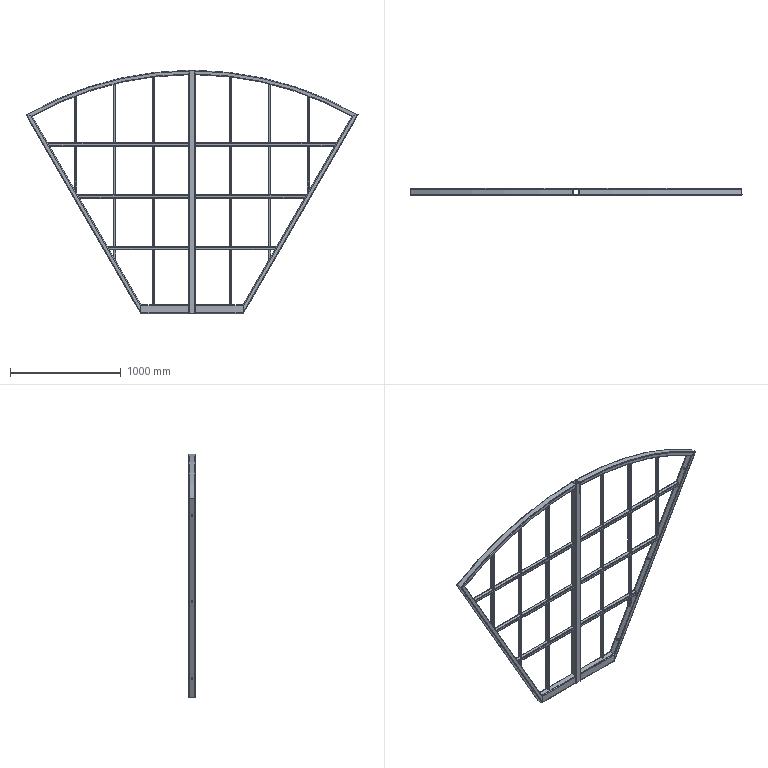Part | SolidWorks | features WeldCornerFeat 7, WeldMemberFeat 5, HoleWzd 2, MirrorPattern 1, MirrorSolid 1, WeldmentFeature 1 | 33 solids | 620 faces | box 3000 x 60 x 2200 mm | volume 10098660 mm3 | plane 316 | cylinder 288 | torus 16 | commonest cylinder face diameters 5 x80 10 x80 6 x36 12 x36 17 x26 8 x8